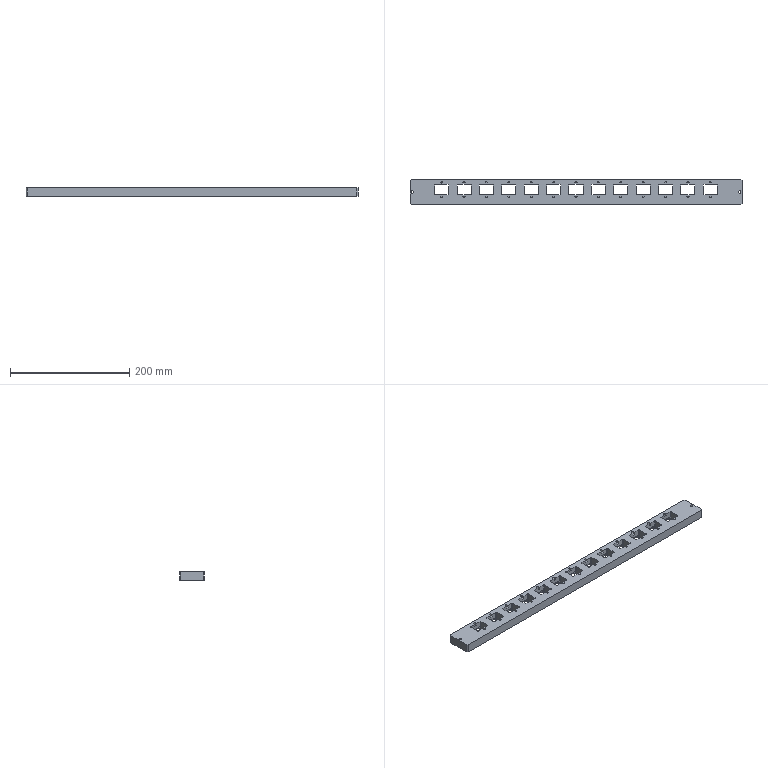NC program | NX | posted with a generic post | part box 556 x 41 x 15 mm
Lines 5367 to 6213 of 52182:
(ZLEVEL_PROFILE_COPY_1_COPY_COPY_2_COPY , TOOL : D2)
N10732 T02 M6
N10734 G54
N10736 G17 G0 G90 X-217.612 Y12.426 S5000 M3
N10738 G43 Z30. H2
N10740 Z-0.04
N10742 G94 G1 X-217.35 Y12.577 F1000.
N10744 G3 X-217.25 Y12.75 R0.2
N10746 G1 Y14.75 F1100.
N10748 X-219.466
N10750 G3 X-219.64 Y14.65 R0.2
N10752 G1 X-219.813 Y14.35
N10754 G0 X-217.612 Y12.426 Z-0.08
N10756 G1 X-217.35 Y12.577 F1000.
N10758 G3 X-217.25 Y12.75 R0.2
N10760 G1 Y14.75 F1100.
N10762 X-219.466
N10764 G3 X-219.64 Y14.65 R0.2
N10766 G1 X-219.813 Y14.35
N10768 G0 X-217.612 Y12.426 Z-0.12
N10770 G1 X-217.35 Y12.577 F1000.
N10772 G3 X-217.25 Y12.75 R0.2
N10774 G1 Y14.75 F1100.
N10776 X-219.466
N10778 G3 X-219.64 Y14.65 R0.2
N10780 G1 X-219.813 Y14.35
N10782 G0 X-217.612 Y12.426 Z-0.16
N10784 G1 X-217.35 Y12.577 F1000.
N10786 G3 X-217.25 Y12.75 R0.2
N10788 G1 Y14.75 F1100.
N10790 X-219.466
N10792 G3 X-219.64 Y14.65 R0.2
N10794 G1 X-219.813 Y14.35
N10796 G0 X-217.612 Y12.426 Z-0.2
N10798 G1 X-217.35 Y12.577 F1000.
N10800 G3 X-217.25 Y12.75 R0.2
N10802 G1 Y14.75 F1100.
N10804 X-219.466
N10806 G3 X-219.64 Y14.65 R0.2
N10808 G1 X-219.813 Y14.35
N10810 G0 X-217.612 Y12.426 Z-0.24
N10812 G1 X-217.35 Y12.577 F1000.
N10814 G3 X-217.25 Y12.75 R0.2
N10816 G1 Y14.75 F1100.
N10818 X-219.466
N10820 G3 X-219.64 Y14.65 R0.2
N10822 G1 X-219.813 Y14.35
N10824 G0 X-217.612 Y12.426 Z-0.28
N10826 G1 X-217.35 Y12.577 F1000.
N10828 G3 X-217.25 Y12.75 R0.2
N10830 G1 Y14.75 F1100.
N10832 X-219.466
N10834 G3 X-219.64 Y14.65 R0.2
N10836 G1 X-219.813 Y14.35
N10838 G0 X-217.612 Y12.426 Z-0.32
N10840 G1 X-217.35 Y12.577 F1000.
N10842 G3 X-217.25 Y12.75 R0.2
N10844 G1 Y14.75 F1100.
N10846 X-219.466
N10848 G3 X-219.64 Y14.65 R0.2
N10850 G1 X-219.813 Y14.35
N10852 G0 X-217.612 Y12.426 Z-0.36
N10854 G1 X-217.35 Y12.577 F1000.
N10856 G3 X-217.25 Y12.75 R0.2
N10858 G1 Y14.75 F1100.
N10860 X-219.466
N10862 G3 X-219.64 Y14.65 R0.2
N10864 G1 X-219.813 Y14.35
N10866 G0 X-217.612 Y12.426 Z-0.4
N10868 G1 X-217.35 Y12.577 F1000.
N10870 G3 X-217.25 Y12.75 R0.2
N10872 G1 Y14.75 F1100.
N10874 X-219.466
N10876 G3 X-219.64 Y14.65 R0.2
N10878 G1 X-219.813 Y14.35
N10880 G0 X-217.612 Y12.426 Z-0.44
N10882 G1 X-217.35 Y12.577 F1000.
N10884 G3 X-217.25 Y12.75 R0.2
N10886 G1 Y14.75 F1100.
N10888 X-219.466
N10890 G3 X-219.64 Y14.65 R0.2
N10892 G1 X-219.813 Y14.35
N10894 G0 X-217.612 Y12.426 Z-0.48
N10896 G1 X-217.35 Y12.577 F1000.
N10898 G3 X-217.25 Y12.75 R0.2
N10900 G1 Y14.75 F1100.
N10902 X-219.466
N10904 G3 X-219.64 Y14.65 R0.2
N10906 G1 X-219.813 Y14.35
N10908 G0 X-217.612 Y12.426 Z-0.52
N10910 G1 X-217.35 Y12.577 F1000.
N10912 G3 X-217.25 Y12.75 R0.2
N10914 G1 Y14.75 F1100.
N10916 X-219.466
N10918 G3 X-219.64 Y14.65 R0.2
N10920 G1 X-219.813 Y14.35
N10922 G0 X-217.612 Y12.426 Z-0.56
N10924 G1 X-217.35 Y12.577 F1000.
N10926 G3 X-217.25 Y12.75 R0.2
N10928 G1 Y14.75 F1100.
N10930 X-219.466
N10932 G3 X-219.64 Y14.65 R0.2
N10934 G1 X-219.813 Y14.35
N10936 G0 X-217.612 Y12.426 Z-0.6
N10938 G1 X-217.35 Y12.577 F1000.
N10940 G3 X-217.25 Y12.75 R0.2
N10942 G1 Y14.75 F1100.
N10944 X-219.466
N10946 G3 X-219.64 Y14.65 R0.2
N10948 G1 X-219.813 Y14.35
N10950 G0 X-217.612 Y12.426 Z-0.64
N10952 G1 X-217.35 Y12.577 F1000.
N10954 G3 X-217.25 Y12.75 R0.2
N10956 G1 Y14.75 F1100.
N10958 X-219.467
N10960 G3 X-219.64 Y14.65 R0.2
N10962 G1 X-219.813 Y14.35
N10964 G0 X-217.612 Y12.426 Z-0.68
N10966 G1 X-217.35 Y12.577 F1000.
N10968 G3 X-217.25 Y12.75 R0.2
N10970 G1 Y14.75 F1100.
N10972 X-219.467
N10974 G3 X-219.64 Y14.65 R0.2
N10976 G1 X-219.813 Y14.35
N10978 G0 X-217.612 Y12.426 Z-0.72
N10980 G1 X-217.35 Y12.577 F1000.
N10982 G3 X-217.25 Y12.75 R0.2
N10984 G1 Y14.75 F1100.
N10986 X-219.467
N10988 G3 X-219.64 Y14.65 R0.2
N10990 G1 X-219.813 Y14.35
N10992 G0 X-217.612 Y12.426 Z-0.76
N10994 G1 X-217.35 Y12.577 F1000.
N10996 G3 X-217.25 Y12.75 R0.2
N10998 G1 Y14.75 F1100.
N11000 X-219.467
N11002 G3 X-219.64 Y14.65 R0.2
N11004 G1 X-219.813 Y14.35
N11006 G0 X-217.612 Y12.426 Z-0.8
N11008 G1 X-217.35 Y12.577 F1000.
N11010 G3 X-217.25 Y12.75 R0.2
N11012 G1 Y14.75 F1100.
N11014 X-219.467
N11016 G3 X-219.64 Y14.65 R0.2
N11018 G1 X-219.813 Y14.35
N11020 G0 X-217.612 Y12.426 Z-0.84
N11022 G1 X-217.35 Y12.577 F1000.
N11024 G3 X-217.25 Y12.75 R0.2
N11026 G1 Y14.75 F1100.
N11028 X-219.467
N11030 G3 X-219.64 Y14.65 R0.2
N11032 G1 X-219.813 Y14.35
N11034 G0 X-217.612 Y12.426 Z-0.88
N11036 G1 X-217.35 Y12.577 F1000.
N11038 G3 X-217.25 Y12.75 R0.2
N11040 G1 Y14.75 F1100.
N11042 X-219.467
N11044 G3 X-219.64 Y14.65 R0.2
N11046 G1 X-219.813 Y14.35
N11048 G0 X-217.612 Y12.426 Z-0.92
N11050 G1 X-217.35 Y12.577 F1000.
N11052 G3 X-217.25 Y12.75 R0.2
N11054 G1 Y14.75 F1100.
N11056 X-219.467
N11058 G3 X-219.64 Y14.65 R0.2
N11060 G1 X-219.813 Y14.35
N11062 G0 X-217.612 Y12.426 Z-0.96
N11064 G1 X-217.35 Y12.577 F1000.
N11066 G3 X-217.25 Y12.75 R0.2
N11068 G1 Y14.75 F1100.
N11070 X-219.467
N11072 G3 X-219.64 Y14.65 R0.2
N11074 G1 X-219.813 Y14.35
N11076 G0 X-217.612 Y12.426 Z-1.
N11078 G1 X-217.35 Y12.577 F1000.
N11080 G3 X-217.25 Y12.75 R0.2
N11082 G1 Y14.75 F1100.
N11084 X-219.467
N11086 G3 X-219.64 Y14.65 R0.2
N11088 G1 X-219.813 Y14.35
N11090 G0 X-217.612 Y12.426 Z-1.04
N11092 G1 X-217.35 Y12.577 F1000.
N11094 G3 X-217.25 Y12.75 R0.2
N11096 G1 Y14.75 F1100.
N11098 X-219.467
N11100 G3 X-219.64 Y14.65 R0.2
N11102 G1 X-219.813 Y14.35
N11104 G0 X-217.612 Y12.426 Z-1.08
N11106 G1 X-217.35 Y12.577 F1000.
N11108 G3 X-217.25 Y12.75 R0.2
N11110 G1 Y14.75 F1100.
N11112 X-219.467
N11114 G3 X-219.64 Y14.65 R0.2
N11116 G1 X-219.813 Y14.35
N11118 G0 X-217.612 Y12.426 Z-1.12
N11120 G1 X-217.35 Y12.577 F1000.
N11122 G3 X-217.25 Y12.75 R0.2
N11124 G1 Y14.75 F1100.
N11126 X-219.467
N11128 G3 X-219.64 Y14.65 R0.2
N11130 G1 X-219.813 Y14.35
N11132 G0 X-217.612 Y12.426 Z-1.16
N11134 G1 X-217.35 Y12.577 F1000.
N11136 G3 X-217.25 Y12.75 R0.2
N11138 G1 Y14.75 F1100.
N11140 X-219.467
N11142 G3 X-219.64 Y14.65 R0.2
N11144 G1 X-219.813 Y14.35
N11146 G0 X-217.612 Y12.426 Z-1.2
N11148 G1 X-217.35 Y12.577 F1000.
N11150 G3 X-217.25 Y12.75 R0.2
N11152 G1 Y14.75 F1100.
N11154 X-219.467
N11156 G3 X-219.64 Y14.65 R0.2
N11158 G1 X-219.813 Y14.35
N11160 G0 X-217.612 Y12.426 Z-1.24
N11162 G1 X-217.35 Y12.577 F1000.
N11164 G3 X-217.25 Y12.75 R0.2
N11166 G1 Y14.75 F1100.
N11168 X-219.467
N11170 G3 X-219.64 Y14.65 R0.2
N11172 G1 X-219.813 Y14.35
N11174 G0 X-217.612 Y12.426 Z-1.28
N11176 G1 X-217.35 Y12.577 F1000.
N11178 G3 X-217.25 Y12.75 R0.2
N11180 G1 Y14.75 F1100.
N11182 X-219.467
N11184 G3 X-219.64 Y14.65 R0.2
N11186 G1 X-219.813 Y14.35
N11188 G0 X-217.612 Y12.426 Z-1.32
N11190 G1 X-217.35 Y12.577 F1000.
N11192 G3 X-217.25 Y12.75 R0.2
N11194 G1 Y14.75 F1100.
N11196 X-219.467
N11198 G3 X-219.64 Y14.65 R0.2
N11200 G1 X-219.813 Y14.35
N11202 G0 X-217.612 Y12.426 Z-1.36
N11204 G1 X-217.35 Y12.577 F1000.
N11206 G3 X-217.25 Y12.75 R0.2
N11208 G1 Y14.75 F1100.
N11210 X-219.467
N11212 G3 X-219.64 Y14.65 R0.2
N11214 G1 X-219.813 Y14.35
N11216 G0 X-217.612 Y12.426 Z-1.4
N11218 G1 X-217.35 Y12.577 F1000.
N11220 G3 X-217.25 Y12.75 R0.2
N11222 G1 Y14.75 F1100.
N11224 X-219.467
N11226 G3 X-219.64 Y14.65 R0.2
N11228 G1 X-219.813 Y14.35
N11230 G0 X-217.612 Y12.426 Z-1.44
N11232 G1 X-217.35 Y12.577 F1000.
N11234 G3 X-217.25 Y12.75 R0.2
N11236 G1 Y14.75 F1100.
N11238 X-219.467
N11240 G3 X-219.64 Y14.65 R0.2
N11242 G1 X-219.813 Y14.35
N11244 G0 X-217.612 Y12.426 Z-1.48
N11246 G1 X-217.35 Y12.577 F1000.
N11248 G3 X-217.25 Y12.75 R0.2
N11250 G1 Y14.75 F1100.
N11252 X-219.467
N11254 G3 X-219.64 Y14.65 R0.2
N11256 G1 X-219.813 Y14.35
N11258 G0 X-217.612 Y12.426 Z-1.52
N11260 G1 X-217.35 Y12.577 F1000.
N11262 G3 X-217.25 Y12.75 R0.2
N11264 G1 Y14.75 F1100.
N11266 X-219.467
N11268 G3 X-219.64 Y14.65 R0.2
N11270 G1 X-219.813 Y14.35
N11272 G0 X-217.612 Y12.426 Z-1.56
N11274 G1 X-217.35 Y12.577 F1000.
N11276 G3 X-217.25 Y12.75 R0.2
N11278 G1 Y14.75 F1100.
N11280 X-219.467
N11282 G3 X-219.64 Y14.65 R0.2
N11284 G1 X-219.813 Y14.35
N11286 G0 X-217.612 Y12.426 Z-1.6
N11288 G1 X-217.35 Y12.577 F1000.
N11290 G3 X-217.25 Y12.75 R0.2
N11292 G1 Y14.75 F1100.
N11294 X-219.467
N11296 G3 X-219.64 Y14.65 R0.2
N11298 G1 X-219.813 Y14.35
N11300 G0 X-217.612 Y12.426 Z-1.64
N11302 G1 X-217.35 Y12.577 F1000.
N11304 G3 X-217.25 Y12.75 R0.2
N11306 G1 Y14.75 F1100.
N11308 X-219.467
N11310 G3 X-219.64 Y14.65 R0.2
N11312 G1 X-219.813 Y14.35
N11314 G0 X-217.612 Y12.426 Z-1.68
N11316 G1 X-217.35 Y12.577 F1000.
N11318 G3 X-217.25 Y12.75 R0.2
N11320 G1 Y14.75 F1100.
N11322 X-219.467
N11324 G3 X-219.64 Y14.65 R0.2
N11326 G1 X-219.813 Y14.35
N11328 G0 X-217.612 Y12.426 Z-1.72
N11330 G1 X-217.35 Y12.577 F1000.
N11332 G3 X-217.25 Y12.75 R0.2
N11334 G1 Y14.75 F1100.
N11336 X-219.467
N11338 G3 X-219.64 Y14.65 R0.2
N11340 G1 X-219.813 Y14.35
N11342 G0 X-217.612 Y12.426 Z-1.76
N11344 G1 X-217.35 Y12.577 F1000.
N11346 G3 X-217.25 Y12.75 R0.2
N11348 G1 Y14.75 F1100.
N11350 X-219.467
N11352 G3 X-219.64 Y14.65 R0.2
N11354 G1 X-219.813 Y14.35
N11356 G0 X-217.612 Y12.426 Z-1.8
N11358 G1 X-217.35 Y12.577 F1000.
N11360 G3 X-217.25 Y12.75 R0.2
N11362 G1 Y14.75 F1100.
N11364 X-219.467
N11366 G3 X-219.64 Y14.65 R0.2
N11368 G1 X-219.813 Y14.35
N11370 G0 X-217.612 Y12.426 Z-1.84
N11372 G1 X-217.35 Y12.577 F1000.
N11374 G3 X-217.25 Y12.75 R0.2
N11376 G1 Y14.75 F1100.
N11378 X-219.467
N11380 G3 X-219.64 Y14.65 R0.2
N11382 G1 X-219.813 Y14.35
N11384 G0 X-217.612 Y12.426 Z-1.88
N11386 G1 X-217.35 Y12.577 F1000.
N11388 G3 X-217.25 Y12.75 R0.2
N11390 G1 Y14.75 F1100.
N11392 X-219.467
N11394 G3 X-219.64 Y14.65 R0.2
N11396 G1 X-219.813 Y14.35
N11398 G0 X-217.612 Y12.426 Z-1.92
N11400 G1 X-217.35 Y12.577 F1000.
N11402 G3 X-217.25 Y12.75 R0.2
N11404 G1 Y14.75 F1100.
N11406 X-219.467
N11408 G3 X-219.64 Y14.65 R0.2
N11410 G1 X-219.813 Y14.35
N11412 G0 X-217.612 Y12.426 Z-1.96
N11414 G1 X-217.35 Y12.577 F1000.
N11416 G3 X-217.25 Y12.75 R0.2
N11418 G1 Y14.75 F1100.
N11420 X-219.467
N11422 G3 X-219.64 Y14.65 R0.2
N11424 G1 X-219.813 Y14.35
N11426 G0 X-217.612 Y12.426 Z-2.
N11428 G1 X-217.35 Y12.577 F1000.
N11430 G3 X-217.25 Y12.75 R0.2
N11432 G1 Y14.75 F1100.
N11434 X-219.467
N11436 G3 X-219.64 Y14.65 R0.2
N11438 G1 X-219.813 Y14.35
N11440 G0 X-217.612 Y12.426 Z-2.04
N11442 G1 X-217.35 Y12.577 F1000.
N11444 G3 X-217.25 Y12.75 R0.2
N11446 G1 Y14.75 F1100.
N11448 X-219.467
N11450 G3 X-219.64 Y14.65 R0.2
N11452 G1 X-219.813 Y14.35
N11454 G0 X-217.612 Y12.426 Z-2.08
N11456 G1 X-217.35 Y12.577 F1000.
N11458 G3 X-217.25 Y12.75 R0.2
N11460 G1 Y14.75 F1100.
N11462 X-219.467
N11464 G3 X-219.64 Y14.65 R0.2
N11466 G1 X-219.813 Y14.35
N11468 G0 X-217.612 Y12.426 Z-2.12
N11470 G1 X-217.35 Y12.577 F1000.
N11472 G3 X-217.25 Y12.75 R0.2
N11474 G1 Y14.75 F1100.
N11476 X-219.467
N11478 G3 X-219.64 Y14.65 R0.2
N11480 G1 X-219.813 Y14.35
N11482 G0 X-217.612 Y12.426 Z-2.16
N11484 G1 X-217.35 Y12.577 F1000.
N11486 G3 X-217.25 Y12.75 R0.2
N11488 G1 Y14.75 F1100.
N11490 X-219.467
N11492 G3 X-219.64 Y14.65 R0.2
N11494 G1 X-219.813 Y14.35
N11496 G0 X-217.612 Y12.426 Z-2.2
N11498 G1 X-217.35 Y12.577 F1000.
N11500 G3 X-217.25 Y12.75 R0.2
N11502 G1 Y14.75 F1100.
N11504 X-219.467
N11506 G3 X-219.64 Y14.65 R0.2
N11508 G1 X-219.813 Y14.35
N11510 G0 X-217.612 Y12.426 Z-2.24
N11512 G1 X-217.35 Y12.577 F1000.
N11514 G3 X-217.25 Y12.75 R0.2
N11516 G1 Y14.75 F1100.
N11518 X-219.467
N11520 G3 X-219.64 Y14.65 R0.2
N11522 G1 X-219.813 Y14.35
N11524 G0 X-217.612 Y12.426 Z-2.28
N11526 G1 X-217.35 Y12.577 F1000.
N11528 G3 X-217.25 Y12.75 R0.2
N11530 G1 Y14.75 F1100.
N11532 X-219.467
N11534 G3 X-219.64 Y14.65 R0.2
N11536 G1 X-219.813 Y14.35
N11538 G0 X-217.612 Y12.426 Z-2.32
N11540 G1 X-217.35 Y12.577 F1000.
N11542 G3 X-217.25 Y12.75 R0.2
N11544 G1 Y14.75 F1100.
N11546 X-219.467
N11548 G3 X-219.64 Y14.65 R0.2
N11550 G1 X-219.813 Y14.35
N11552 G0 X-217.612 Y12.426 Z-2.36
N11554 G1 X-217.35 Y12.577 F1000.
N11556 G3 X-217.25 Y12.75 R0.2
N11558 G1 Y14.75 F1100.
N11560 X-219.467
N11562 G3 X-219.64 Y14.65 R0.2
N11564 G1 X-219.813 Y14.35
N11566 G0 X-217.612 Y12.426 Z-2.4
N11568 G1 X-217.35 Y12.577 F1000.
N11570 G3 X-217.25 Y12.75 R0.2
N11572 G1 Y14.75 F1100.
N11574 X-219.467
N11576 G3 X-219.64 Y14.65 R0.2
N11578 G1 X-219.813 Y14.35
N11580 G0 X-217.612 Y12.426 Z-2.44
N11582 G1 X-217.35 Y12.577 F1000.
N11584 G3 X-217.25 Y12.75 R0.2
N11586 G1 Y14.75 F1100.
N11588 X-219.467
N11590 G3 X-219.64 Y14.65 R0.2
N11592 G1 X-219.813 Y14.35
N11594 G0 X-217.612 Y12.426 Z-2.48
N11596 G1 X-217.35 Y12.577 F1000.
N11598 G3 X-217.25 Y12.75 R0.2
N11600 G1 Y14.75 F1100.
N11602 X-219.467
N11604 G3 X-219.64 Y14.65 R0.2
N11606 G1 X-219.813 Y14.35
N11608 G0 X-217.612 Y12.426 Z-2.52
N11610 G1 X-217.35 Y12.577 F1000.
N11612 G3 X-217.25 Y12.75 R0.2
N11614 G1 Y14.75 F1100.
N11616 X-219.467
N11618 G3 X-219.64 Y14.65 R0.2
N11620 G1 X-219.813 Y14.35
N11622 G0 X-217.612 Y12.426 Z-2.56
N11624 G1 X-217.35 Y12.577 F1000.
N11626 G3 X-217.25 Y12.75 R0.2
N11628 G1 Y14.75 F1100.
N11630 X-219.467
N11632 G3 X-219.64 Y14.65 R0.2
N11634 G1 X-219.813 Y14.35
N11636 G0 X-217.612 Y12.426 Z-2.6
N11638 G1 X-217.35 Y12.577 F1000.
N11640 G3 X-217.25 Y12.75 R0.2
N11642 G1 Y14.75 F1100.
N11644 X-219.467
N11646 G3 X-219.64 Y14.65 R0.2
N11648 G1 X-219.813 Y14.35
N11650 G0 X-217.612 Y12.426 Z-2.64
N11652 G1 X-217.35 Y12.577 F1000.
N11654 G3 X-217.25 Y12.75 R0.2
N11656 G1 Y14.75 F1100.
N11658 X-219.467
N11660 G3 X-219.64 Y14.65 R0.2
N11662 G1 X-219.813 Y14.35
N11664 G0 X-217.612 Y12.426 Z-2.68
N11666 G1 X-217.35 Y12.577 F1000.
N11668 G3 X-217.25 Y12.75 R0.2
N11670 G1 Y14.75 F1100.
N11672 X-219.467
N11674 G3 X-219.64 Y14.65 R0.2
N11676 G1 X-219.813 Y14.35
N11678 G0 X-217.612 Y12.426 Z-2.72
N11680 G1 X-217.35 Y12.577 F1000.
N11682 G3 X-217.25 Y12.75 R0.2
N11684 G1 Y14.75 F1100.
N11686 X-219.467
N11688 G3 X-219.64 Y14.65 R0.2
N11690 G1 X-219.813 Y14.35
N11692 G0 X-217.612 Y12.426 Z-2.76
N11694 G1 X-217.35 Y12.577 F1000.
N11696 G3 X-217.25 Y12.75 R0.2
N11698 G1 Y14.75 F1100.
N11700 X-219.467
N11702 G3 X-219.64 Y14.65 R0.2
N11704 G1 X-219.813 Y14.35
N11706 G0 X-217.612 Y12.426 Z-2.8
N11708 G1 X-217.35 Y12.577 F1000.
N11710 G3 X-217.25 Y12.75 R0.2
N11712 G1 Y14.75 F1100.
N11714 X-219.467
N11716 G3 X-219.64 Y14.65 R0.2
N11718 G1 X-219.813 Y14.35
N11720 G0 X-217.612 Y12.426 Z-2.84
N11722 G1 X-217.35 Y12.577 F1000.
N11724 G3 X-217.25 Y12.75 R0.2
N11726 G1 Y14.75 F1100.
N11728 X-219.467
N11730 G3 X-219.64 Y14.65 R0.2
N11732 G1 X-219.813 Y14.35
N11734 G0 X-217.612 Y12.426 Z-2.88
N11736 G1 X-217.35 Y12.577 F1000.
N11738 G3 X-217.25 Y12.75 R0.2
N11740 G1 Y14.75 F1100.
N11742 X-219.467
N11744 G3 X-219.64 Y14.65 R0.2
N11746 G1 X-219.813 Y14.35
N11748 G0 X-217.612 Y12.426 Z-2.92
N11750 G1 X-217.35 Y12.577 F1000.
N11752 G3 X-217.25 Y12.75 R0.2
N11754 G1 Y14.75 F1100.
N11756 X-219.467
N11758 G3 X-219.64 Y14.65 R0.2
N11760 G1 X-219.813 Y14.35
N11762 G0 X-217.612 Y12.426 Z-2.96
N11764 G1 X-217.35 Y12.577 F1000.
N11766 G3 X-217.25 Y12.75 R0.2
N11768 G1 Y14.75 F1100.
N11770 X-219.467
N11772 G3 X-219.64 Y14.65 R0.2
N11774 G1 X-219.813 Y14.35
N11776 G0 X-217.612 Y12.426 Z-3.
N11778 G1 X-217.35 Y12.577 F1000.
N11780 G3 X-217.25 Y12.75 R0.2
N11782 G1 Y14.75 F1100.
N11784 X-219.467
N11786 G3 X-219.64 Y14.65 R0.2
N11788 G1 X-219.813 Y14.35
N11790 G0 X-217.612 Y12.426 Z-3.04
N11792 G1 X-217.35 Y12.577 F1000.
N11794 G3 X-217.25 Y12.75 R0.2
N11796 G1 Y14.75 F1100.
N11798 X-219.467
N11800 G3 X-219.64 Y14.65 R0.2
N11802 G1 X-219.813 Y14.35
N11804 G0 X-217.612 Y12.426 Z-3.08
N11806 G1 X-217.35 Y12.577 F1000.
N11808 G3 X-217.25 Y12.75 R0.2
N11810 G1 Y14.75 F1100.
N11812 X-219.467
N11814 G3 X-219.64 Y14.65 R0.2
N11816 G1 X-219.813 Y14.35
N11818 G0 X-217.612 Y12.426 Z-3.12
N11820 G1 X-217.35 Y12.577 F1000.
N11822 G3 X-217.25 Y12.75 R0.2
N11824 G1 Y14.75 F1100.
N11826 X-219.467
N11828 G3 X-219.64 Y14.65 R0.2
N11830 G1 X-219.813 Y14.35
N11832 G0 X-217.612 Y12.426 Z-3.16
N11834 G1 X-217.35 Y12.577 F1000.
N11836 G3 X-217.25 Y12.75 R0.2
N11838 G1 Y14.75 F1100.
N11840 X-219.467
N11842 G3 X-219.64 Y14.65 R0.2
N11844 G1 X-219.813 Y14.35
N11846 G0 X-217.612 Y12.426 Z-3.2
N11848 G1 X-217.35 Y12.577 F1000.
N11850 G3 X-217.25 Y12.75 R0.2
N11852 G1 Y14.75 F1100.
N11854 X-219.467
N11856 G3 X-219.64 Y14.65 R0.2
N11858 G1 X-219.813 Y14.35
N11860 G0 X-217.612 Y12.426 Z-3.24
N11862 G1 X-217.35 Y12.577 F1000.
N11864 G3 X-217.25 Y12.75 R0.2
N11866 G1 Y14.75 F1100.
N11868 X-219.467
N11870 G3 X-219.64 Y14.65 R0.2
N11872 G1 X-219.813 Y14.35
N11874 G0 X-217.612 Y12.426 Z-3.28
N11876 G1 X-217.35 Y12.577 F1000.
N11878 G3 X-217.25 Y12.75 R0.2
N11880 G1 Y14.75 F1100.
N11882 X-219.467
N11884 G3 X-219.64 Y14.65 R0.2
N11886 G1 X-219.813 Y14.35
N11888 G0 X-217.612 Y12.426 Z-3.32
N11890 G1 X-217.35 Y12.577 F1000.
N11892 G3 X-217.25 Y12.75 R0.2
N11894 G1 Y14.75 F1100.
N11896 X-219.467
N11898 G3 X-219.64 Y14.65 R0.2
N11900 G1 X-219.813 Y14.35
N11902 G0 X-217.612 Y12.426 Z-3.36
N11904 G1 X-217.35 Y12.577 F1000.
N11906 G3 X-217.25 Y12.75 R0.2
N11908 G1 Y14.75 F1100.
N11910 X-219.467
N11912 G3 X-219.64 Y14.65 R0.2
N11914 G1 X-219.813 Y14.35
N11916 G0 X-217.612 Y12.426 Z-3.4
N11918 G1 X-217.35 Y12.577 F1000.
N11920 G3 X-217.25 Y12.75 R0.2
N11922 G1 Y14.75 F1100.
N11924 X-219.467
N11926 G3 X-219.64 Y14.65 R0.2
N11928 G1 X-219.813 Y14.35
N11930 G0 X-217.612 Y12.426 Z-3.44
N11932 G1 X-217.35 Y12.577 F1000.
N11934 G3 X-217.25 Y12.75 R0.2
N11936 G1 Y14.75 F1100.
N11938 X-219.467
N11940 G3 X-219.64 Y14.65 R0.2
N11942 G1 X-219.813 Y14.35
N11944 G0 X-217.612 Y12.426 Z-3.48
N11946 G1 X-217.35 Y12.577 F1000.
N11948 G3 X-217.25 Y12.75 R0.2
N11950 G1 Y14.75 F1100.
N11952 X-219.467
N11954 G3 X-219.64 Y14.65 R0.2
N11956 G1 X-219.813 Y14.35
N11958 G0 X-217.612 Y12.426 Z-3.52
N11960 G1 X-217.35 Y12.577 F1000.
N11962 G3 X-217.25 Y12.75 R0.2
N11964 G1 Y14.75 F1100.
N11966 X-219.467
N11968 G3 X-219.64 Y14.65 R0.2
N11970 G1 X-219.813 Y14.35
N11972 G0 X-217.612 Y12.426 Z-3.56
N11974 G1 X-217.35 Y12.577 F1000.
N11976 G3 X-217.25 Y12.75 R0.2
N11978 G1 Y14.75 F1100.
N11980 X-219.467
N11982 G3 X-219.64 Y14.65 R0.2
N11984 G1 X-219.813 Y14.35
N11986 G0 X-217.612 Y12.426 Z-3.6
N11988 G1 X-217.35 Y12.577 F1000.
N11990 G3 X-217.25 Y12.75 R0.2
N11992 G1 Y14.75 F1100.
N11994 X-219.467
N11996 G3 X-219.64 Y14.65 R0.2
N11998 G1 X-219.813 Y14.35
N12000 G0 X-217.612 Y12.426 Z-3.64
N12002 G1 X-217.35 Y12.577 F1000.
N12004 G3 X-217.25 Y12.75 R0.2
N12006 G1 Y14.75 F1100.
N12008 X-219.467
N12010 G3 X-219.64 Y14.65 R0.2
N12012 G1 X-219.813 Y14.35
N12014 G0 X-217.612 Y12.426 Z-3.68
N12016 G1 X-217.35 Y12.577 F1000.
N12018 G3 X-217.25 Y12.75 R0.2
N12020 G1 Y14.75 F1100.
N12022 X-219.467
N12024 G3 X-219.64 Y14.65 R0.2
N12026 G1 X-219.813 Y14.35
N12028 G0 X-217.612 Y12.426 Z-3.72
N12030 G1 X-217.35 Y12.577 F1000.
N12032 G3 X-217.25 Y12.75 R0.2
N12034 G1 Y14.75 F1100.
N12036 X-219.467
N12038 G3 X-219.64 Y14.65 R0.2
N12040 G1 X-219.813 Y14.35
N12042 G0 X-217.612 Y12.426 Z-3.76
N12044 G1 X-217.35 Y12.577 F1000.
N12046 G3 X-217.25 Y12.75 R0.2
N12048 G1 Y14.75 F1100.
N12050 X-219.467
N12052 G3 X-219.64 Y14.65 R0.2
N12054 G1 X-219.813 Y14.35
N12056 G0 X-217.612 Y12.426 Z-3.8
N12058 G1 X-217.35 Y12.577 F1000.
N12060 G3 X-217.25 Y12.75 R0.2
N12062 G1 Y14.75 F1100.
N12064 X-219.467
N12066 G3 X-219.64 Y14.65 R0.2
N12068 G1 X-219.813 Y14.35
N12070 G0 X-217.612 Y12.426 Z-3.84
N12072 G1 X-217.35 Y12.577 F1000.
N12074 G3 X-217.25 Y12.75 R0.2
N12076 G1 Y14.75 F1100.
N12078 X-219.467
N12080 G3 X-219.64 Y14.65 R0.2
N12082 G1 X-219.813 Y14.35
N12084 G0 X-217.612 Y12.426 Z-3.88
N12086 G1 X-217.35 Y12.577 F1000.
N12088 G3 X-217.25 Y12.75 R0.2
N12090 G1 Y14.75 F1100.
N12092 X-219.467
N12094 G3 X-219.64 Y14.65 R0.2
N12096 G1 X-219.813 Y14.35
N12098 G0 X-217.612 Y12.426 Z-3.92
N12100 G1 X-217.35 Y12.577 F1000.
N12102 G3 X-217.25 Y12.75 R0.2
N12104 G1 Y14.75 F1100.
N12106 X-219.467
N12108 G3 X-219.64 Y14.65 R0.2
N12110 G1 X-219.813 Y14.35
N12112 G0 X-217.612 Y12.426 Z-3.96
N12114 G1 X-217.35 Y12.577 F1000.
N12116 G3 X-217.25 Y12.75 R0.2
N12118 G1 Y14.75 F1100.
N12120 X-219.467
N12122 G3 X-219.64 Y14.65 R0.2
N12124 G1 X-219.813 Y14.35
N12126 G0 X-217.612 Y12.426 Z-4.
N12128 G1 X-217.35 Y12.577 F1000.
N12130 G3 X-217.25 Y12.75 R0.2
N12132 G1 Y14.75 F1100.
N12134 X-219.467
N12136 G3 X-219.64 Y14.65 R0.2
N12138 G1 X-219.813 Y14.35
N12140 G0 X-217.612 Y12.426 Z-4.04
N12142 G1 X-217.35 Y12.577 F1000.
N12144 G3 X-217.25 Y12.75 R0.2
N12146 G1 Y14.75 F1100.
N12148 X-219.467
N12150 G3 X-219.64 Y14.65 R0.2
N12152 G1 X-219.813 Y14.35
N12154 G0 X-217.612 Y12.426 Z-4.08
N12156 G1 X-217.35 Y12.577 F1000.
N12158 G3 X-217.25 Y12.75 R0.2
N12160 G1 Y14.75 F1100.
N12162 X-219.467
N12164 G3 X-219.64 Y14.65 R0.2
N12166 G1 X-219.813 Y14.35
N12168 G0 X-217.612 Y12.426 Z-4.12
N12170 G1 X-217.35 Y12.577 F1000.
N12172 G3 X-217.25 Y12.75 R0.2
N12174 G1 Y14.75 F1100.
N12176 X-219.467
N12178 G3 X-219.64 Y14.65 R0.2
N12180 G1 X-219.813 Y14.35
N12182 G0 X-217.612 Y12.426 Z-4.16
N12184 G1 X-217.35 Y12.577 F1000.
N12186 G3 X-217.25 Y12.75 R0.2
N12188 G1 Y14.75 F1100.
N12190 X-219.467
N12192 G3 X-219.64 Y14.65 R0.2
N12194 G1 X-219.813 Y14.35
N12196 G0 X-217.612 Y12.426 Z-4.2
N12198 G1 X-217.35 Y12.577 F1000.
N12200 G3 X-217.25 Y12.75 R0.2
N12202 G1 Y14.75 F1100.
N12204 X-219.467
N12206 G3 X-219.64 Y14.65 R0.2
N12208 G1 X-219.813 Y14.35
N12210 G0 X-217.612 Y12.426 Z-4.24
N12212 G1 X-217.35 Y12.577 F1000.
N12214 G3 X-217.25 Y12.75 R0.2
N12216 G1 Y14.75 F1100.
N12218 X-219.467
N12220 G3 X-219.64 Y14.65 R0.2
N12222 G1 X-219.813 Y14.35
N12224 G0 X-217.612 Y12.426 Z-4.28
N12226 G1 X-217.35 Y12.577 F1000.
N12228 G3 X-217.25 Y12.75 R0.2
N12230 G1 Y14.75 F1100.
N12232 X-219.467
N12234 G3 X-219.64 Y14.65 R0.2
N12236 G1 X-219.813 Y14.35
N12238 G0 X-217.612 Y12.426 Z-4.32
N12240 G1 X-217.35 Y12.577 F1000.
N12242 G3 X-217.25 Y12.75 R0.2
N12244 G1 Y14.75 F1100.
N12246 X-219.467
N12248 G3 X-219.64 Y14.65 R0.2
N12250 G1 X-219.813 Y14.35
N12252 G0 X-217.612 Y12.426 Z-4.36
N12254 G1 X-217.35 Y12.577 F1000.
N12256 G3 X-217.25 Y12.75 R0.2
N12258 G1 Y14.75 F1100.
N12260 X-219.467
N12262 G3 X-219.64 Y14.65 R0.2
N12264 G1 X-219.813 Y14.35
N12266 G0 X-217.612 Y12.426 Z-4.4
N12268 G1 X-217.35 Y12.577 F1000.
N12270 G3 X-217.25 Y12.75 R0.2
N12272 G1 Y14.75 F1100.
N12274 X-219.467
N12276 G3 X-219.64 Y14.65 R0.2
N12278 G1 X-219.813 Y14.35
N12280 G0 X-217.612 Y12.426 Z-4.44
N12282 G1 X-217.35 Y12.577 F1000.
N12284 G3 X-217.25 Y12.75 R0.2
N12286 G1 Y14.75 F1100.
N12288 X-219.467
N12290 G3 X-219.64 Y14.65 R0.2
N12292 G1 X-219.813 Y14.35
N12294 G0 X-217.612 Y12.426 Z-4.48
N12296 G1 X-217.35 Y12.577 F1000.
N12298 G3 X-217.25 Y12.75 R0.2
N12300 G1 Y14.75 F1100.
N12302 X-219.467
N12304 G3 X-219.64 Y14.65 R0.2
N12306 G1 X-219.813 Y14.35
N12308 G0 X-217.612 Y12.426 Z-4.52
N12310 G1 X-217.35 Y12.577 F1000.
N12312 G3 X-217.25 Y12.75 R0.2
N12314 G1 Y14.75 F1100.
N12316 X-219.467
N12318 G3 X-219.64 Y14.65 R0.2
N12320 G1 X-219.813 Y14.35
N12322 G0 X-217.612 Y12.426 Z-4.56
N12324 G1 X-217.35 Y12.577 F1000.
N12326 G3 X-217.25 Y12.75 R0.2
N12328 G1 Y14.75 F1100.
N12330 X-219.467
N12332 G3 X-219.64 Y14.65 R0.2
N12334 G1 X-219.813 Y14.35
N12336 G0 X-217.612 Y12.426 Z-4.6
N12338 G1 X-217.35 Y12.577 F1000.
N12340 G3 X-217.25 Y12.75 R0.2
N12342 G1 Y14.75 F1100.
N12344 X-219.467
N12346 G3 X-219.64 Y14.65 R0.2
N12348 G1 X-219.813 Y14.35
N12350 G0 X-217.612 Y12.426 Z-4.64
N12352 G1 X-217.35 Y12.577 F1000.
N12354 G3 X-217.25 Y12.75 R0.2
N12356 G1 Y14.75 F1100.
N12358 X-219.467
N12360 G3 X-219.64 Y14.65 R0.2
N12362 G1 X-219.813 Y14.35
N12364 G0 X-217.612 Y12.426 Z-4.68
N12366 G1 X-217.35 Y12.577 F1000.
N12368 G3 X-217.25 Y12.75 R0.2
N12370 G1 Y14.75 F1100.
N12372 X-219.467
N12374 G3 X-219.64 Y14.65 R0.2
N12376 G1 X-219.813 Y14.35
N12378 G0 X-217.612 Y12.426 Z-4.72
N12380 G1 X-217.35 Y12.577 F1000.
N12382 G3 X-217.25 Y12.75 R0.2
N12384 G1 Y14.75 F1100.
N12386 X-219.467
N12388 G3 X-219.64 Y14.65 R0.2
N12390 G1 X-219.813 Y14.35
N12392 G0 X-217.612 Y12.426 Z-4.76
N12394 G1 X-217.35 Y12.577 F1000.
N12396 G3 X-217.25 Y12.75 R0.2
N12398 G1 Y14.75 F1100.
N12400 X-219.467
N12402 G3 X-219.64 Y14.65 R0.2
N12404 G1 X-219.813 Y14.35
N12406 G0 X-217.612 Y12.426 Z-4.8
N12408 G1 X-217.35 Y12.577 F1000.
N12410 G3 X-217.25 Y12.75 R0.2
N12412 G1 Y14.75 F1100.
N12414 X-219.467
N12416 G3 X-219.64 Y14.65 R0.2
N12418 G1 X-219.813 Y14.35